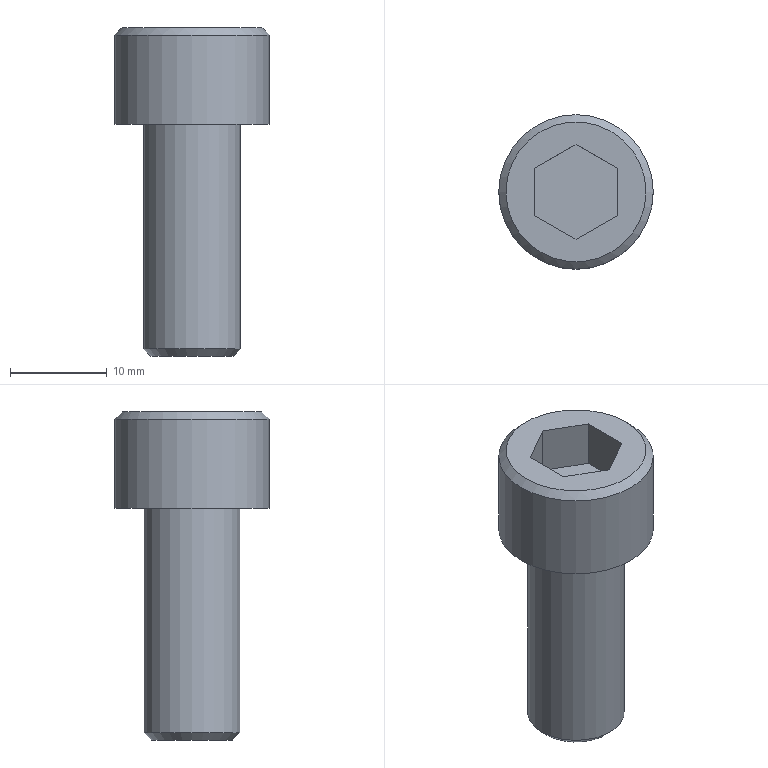Part | STEP file | M10.00-25.00 | 1 solid | 14 faces | box 16 x 16 x 34 mm | volume 3561 mm3 | plane 10 | cylinder 2 | cone 2 | commonest cylinder face diameters 10 x1 16 x1